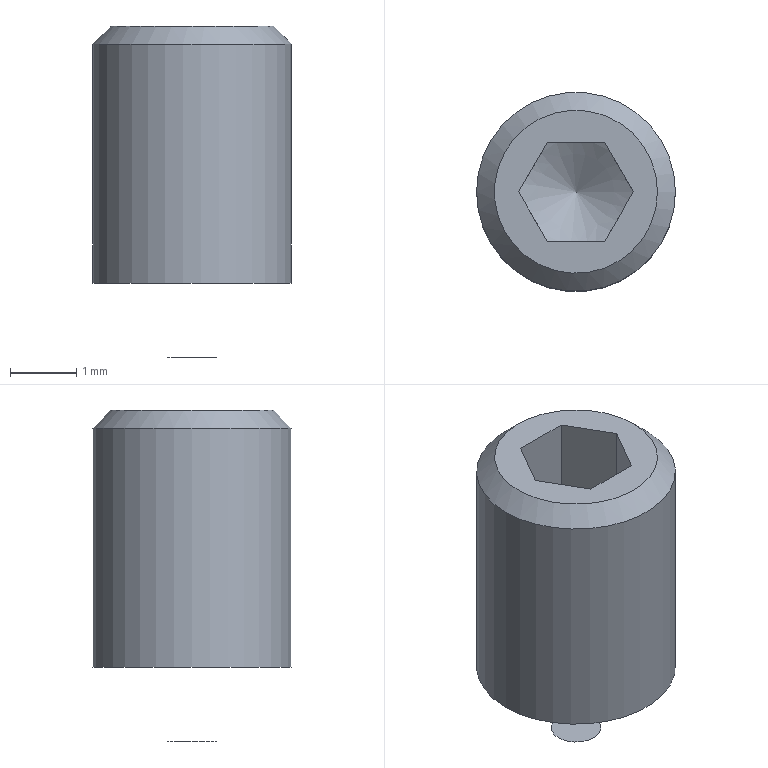Part | NX | features BREP 1, DATUM_CSYS 1 | 1 solid | 12 faces | box 3 x 3 x 5 mm | volume 26.266 mm3 | plane 8 | cone 3 | cylinder 1 | commonest cylinder face diameters 3 x1
STEP:
#1=CARTESIAN_POINT('',(0.866,0.,0.));
#2=VERTEX_POINT('',#1);
#3=CARTESIAN_POINT('',(0.866,0.,-2.));
#4=VERTEX_POINT('',#3);
#5=CARTESIAN_POINT('',(0.866,0.,0.));
#6=DIRECTION('',(0.,0.,-1.));
#7=VECTOR('',#6,1000.);
#8=LINE('',#5,#7);
#9=EDGE_CURVE('',#2,#4,#8,.T.);
#10=ORIENTED_EDGE('',*,*,#9,.T.);
#11=CARTESIAN_POINT('',(0.433,-0.75,-2.));
#12=VERTEX_POINT('',#11);
#13=CARTESIAN_POINT('',(0.866,0.,-2.));
#14=CARTESIAN_POINT('',(0.6495,-0.375,-2.125));
#15=CARTESIAN_POINT('',(0.433,-0.75,-2.));
#16=(BOUNDED_CURVE()B_SPLINE_CURVE(2,(#13,#14,#15),.UNSPECIFIED.,.F.,.F.)B_SPLINE_CURVE_WITH_KNOTS((3,3),(0.,1.),.PIECEWISE_BEZIER_KNOTS.)CURVE()GEOMETRIC_REPRESENTATION_ITEM()RATIONAL_B_SPLINE_CURVE((1.,1.155,1.))REPRESENTATION_ITEM(''));
#17=EDGE_CURVE('',#4,#12,#16,.T.);
#18=ORIENTED_EDGE('',*,*,#17,.T.);
#19=CARTESIAN_POINT('',(0.433,-0.75,0.));
#20=VERTEX_POINT('',#19);
#21=CARTESIAN_POINT('',(0.433,-0.75,0.));
#22=DIRECTION('',(0.,0.,-1.));
#23=VECTOR('',#22,1000.);
#24=LINE('',#21,#23);
#25=EDGE_CURVE('',#20,#12,#24,.T.);
#26=ORIENTED_EDGE('',*,*,#25,.F.);
#27=CARTESIAN_POINT('',(0.866,0.,0.));
#28=DIRECTION('',(-0.5,-0.866,0.));
#29=VECTOR('',#28,1000.);
#30=LINE('',#27,#29);
#31=EDGE_CURVE('',#2,#20,#30,.T.);
#32=ORIENTED_EDGE('',*,*,#31,.F.);
#33=EDGE_LOOP('',(#10,#18,#26,#32));
#34=FACE_BOUND('',#33,.T.);
#35=CARTESIAN_POINT('',(0.6495,-0.375,-1.1));
#36=DIRECTION('',(0.866,-0.5,0.));
#37=DIRECTION('',(0.5,0.866,0.));
#38=AXIS2_PLACEMENT_3D('',#35,#36,#37);
#39=PLANE('',#38);
#40=ADVANCED_FACE('',(#34),#39,.F.);
#41=ORIENTED_EDGE('',*,*,#25,.T.);
#42=CARTESIAN_POINT('',(-0.433,-0.75,-2.));
#43=VERTEX_POINT('',#42);
#44=CARTESIAN_POINT('',(0.433,-0.75,-2.));
#45=CARTESIAN_POINT('',(0.,-0.75,-2.125));
#46=CARTESIAN_POINT('',(-0.433,-0.75,-2.));
#47=(BOUNDED_CURVE()B_SPLINE_CURVE(2,(#44,#45,#46),.UNSPECIFIED.,.F.,.F.)B_SPLINE_CURVE_WITH_KNOTS((3,3),(0.,1.),.PIECEWISE_BEZIER_KNOTS.)CURVE()GEOMETRIC_REPRESENTATION_ITEM()RATIONAL_B_SPLINE_CURVE((1.,1.155,1.))REPRESENTATION_ITEM(''));
#48=EDGE_CURVE('',#12,#43,#47,.T.);
#49=ORIENTED_EDGE('',*,*,#48,.T.);
#50=CARTESIAN_POINT('',(-0.433,-0.75,0.));
#51=VERTEX_POINT('',#50);
#52=CARTESIAN_POINT('',(-0.433,-0.75,0.));
#53=DIRECTION('',(0.,0.,-1.));
#54=VECTOR('',#53,1000.);
#55=LINE('',#52,#54);
#56=EDGE_CURVE('',#51,#43,#55,.T.);
#57=ORIENTED_EDGE('',*,*,#56,.F.);
#58=CARTESIAN_POINT('',(0.433,-0.75,0.));
#59=DIRECTION('',(-1.,0.,0.));
#60=VECTOR('',#59,1000.);
#61=LINE('',#58,#60);
#62=EDGE_CURVE('',#20,#51,#61,.T.);
#63=ORIENTED_EDGE('',*,*,#62,.F.);
#64=EDGE_LOOP('',(#41,#49,#57,#63));
#65=FACE_BOUND('',#64,.T.);
#66=CARTESIAN_POINT('',(0.,-0.75,-1.1));
#67=DIRECTION('',(0.,-1.,0.));
#68=DIRECTION('',(1.,0.,0.));
#69=AXIS2_PLACEMENT_3D('',#66,#67,#68);
#70=PLANE('',#69);
#71=ADVANCED_FACE('',(#65),#70,.F.);
#72=ORIENTED_EDGE('',*,*,#56,.T.);
#73=CARTESIAN_POINT('',(-0.866,0.,-2.));
#74=VERTEX_POINT('',#73);
#75=CARTESIAN_POINT('',(-0.433,-0.75,-2.));
#76=CARTESIAN_POINT('',(-0.6495,-0.375,-2.125));
#77=CARTESIAN_POINT('',(-0.866,0.,-2.));
#78=(BOUNDED_CURVE()B_SPLINE_CURVE(2,(#75,#76,#77),.UNSPECIFIED.,.F.,.F.)B_SPLINE_CURVE_WITH_KNOTS((3,3),(0.,1.),.PIECEWISE_BEZIER_KNOTS.)CURVE()GEOMETRIC_REPRESENTATION_ITEM()RATIONAL_B_SPLINE_CURVE((1.,1.155,1.))REPRESENTATION_ITEM(''));
#79=EDGE_CURVE('',#43,#74,#78,.T.);
#80=ORIENTED_EDGE('',*,*,#79,.T.);
#81=CARTESIAN_POINT('',(-0.866,0.,0.));
#82=VERTEX_POINT('',#81);
#83=CARTESIAN_POINT('',(-0.866,0.,0.));
#84=DIRECTION('',(0.,0.,-1.));
#85=VECTOR('',#84,1000.);
#86=LINE('',#83,#85);
#87=EDGE_CURVE('',#82,#74,#86,.T.);
#88=ORIENTED_EDGE('',*,*,#87,.F.);
#89=CARTESIAN_POINT('',(-0.433,-0.75,0.));
#90=DIRECTION('',(-0.5,0.866,0.));
#91=VECTOR('',#90,1000.);
#92=LINE('',#89,#91);
#93=EDGE_CURVE('',#51,#82,#92,.T.);
#94=ORIENTED_EDGE('',*,*,#93,.F.);
#95=EDGE_LOOP('',(#72,#80,#88,#94));
#96=FACE_BOUND('',#95,.T.);
#97=CARTESIAN_POINT('',(-0.6495,-0.375,-1.1));
#98=DIRECTION('',(-0.866,-0.5,0.));
#99=DIRECTION('',(0.5,-0.866,0.));
#100=AXIS2_PLACEMENT_3D('',#97,#98,#99);
#101=PLANE('',#100);
#102=ADVANCED_FACE('',(#96),#101,.F.);
#103=ORIENTED_EDGE('',*,*,#87,.T.);
#104=CARTESIAN_POINT('',(-0.433,0.75,-2.));
#105=VERTEX_POINT('',#104);
#106=CARTESIAN_POINT('',(-0.866,0.,-2.));
#107=CARTESIAN_POINT('',(-0.6495,0.375,-2.125));
#108=CARTESIAN_POINT('',(-0.433,0.75,-2.));
#109=(BOUNDED_CURVE()B_SPLINE_CURVE(2,(#106,#107,#108),.UNSPECIFIED.,.F.,.F.)B_SPLINE_CURVE_WITH_KNOTS((3,3),(0.,1.),.PIECEWISE_BEZIER_KNOTS.)CURVE()GEOMETRIC_REPRESENTATION_ITEM()RATIONAL_B_SPLINE_CURVE((1.,1.155,1.))REPRESENTATION_ITEM(''));
#110=EDGE_CURVE('',#74,#105,#109,.T.);
#111=ORIENTED_EDGE('',*,*,#110,.T.);
#112=CARTESIAN_POINT('',(-0.433,0.75,0.));
#113=VERTEX_POINT('',#112);
#114=CARTESIAN_POINT('',(-0.433,0.75,0.));
#115=DIRECTION('',(0.,0.,-1.));
#116=VECTOR('',#115,1000.);
#117=LINE('',#114,#116);
#118=EDGE_CURVE('',#113,#105,#117,.T.);
#119=ORIENTED_EDGE('',*,*,#118,.F.);
#120=CARTESIAN_POINT('',(-0.866,0.,0.));
#121=DIRECTION('',(0.5,0.866,0.));
#122=VECTOR('',#121,1000.);
#123=LINE('',#120,#122);
#124=EDGE_CURVE('',#82,#113,#123,.T.);
#125=ORIENTED_EDGE('',*,*,#124,.F.);
#126=EDGE_LOOP('',(#103,#111,#119,#125));
#127=FACE_BOUND('',#126,.T.);
#128=CARTESIAN_POINT('',(-0.6495,0.375,-1.1));
#129=DIRECTION('',(-0.866,0.5,0.));
#130=DIRECTION('',(-0.5,-0.866,0.));
#131=AXIS2_PLACEMENT_3D('',#128,#129,#130);
#132=PLANE('',#131);
#133=ADVANCED_FACE('',(#127),#132,.F.);
#134=ORIENTED_EDGE('',*,*,#118,.T.);
#135=CARTESIAN_POINT('',(0.433,0.75,-2.));
#136=VERTEX_POINT('',#135);
#137=CARTESIAN_POINT('',(-0.433,0.75,-2.));
#138=CARTESIAN_POINT('',(0.,0.75,-2.125));
#139=CARTESIAN_POINT('',(0.433,0.75,-2.));
#140=(BOUNDED_CURVE()B_SPLINE_CURVE(2,(#137,#138,#139),.UNSPECIFIED.,.F.,.F.)B_SPLINE_CURVE_WITH_KNOTS((3,3),(0.,1.),.PIECEWISE_BEZIER_KNOTS.)CURVE()GEOMETRIC_REPRESENTATION_ITEM()RATIONAL_B_SPLINE_CURVE((1.,1.155,1.))REPRESENTATION_ITEM(''));
#141=EDGE_CURVE('',#105,#136,#140,.T.);
#142=ORIENTED_EDGE('',*,*,#141,.T.);
#143=CARTESIAN_POINT('',(0.433,0.75,0.));
#144=VERTEX_POINT('',#143);
#145=CARTESIAN_POINT('',(0.433,0.75,0.));
#146=DIRECTION('',(0.,0.,-1.));
#147=VECTOR('',#146,1000.);
#148=LINE('',#145,#147);
#149=EDGE_CURVE('',#144,#136,#148,.T.);
#150=ORIENTED_EDGE('',*,*,#149,.F.);
#151=CARTESIAN_POINT('',(-0.433,0.75,0.));
#152=DIRECTION('',(1.,0.,0.));
#153=VECTOR('',#152,1000.);
#154=LINE('',#151,#153);
#155=EDGE_CURVE('',#113,#144,#154,.T.);
#156=ORIENTED_EDGE('',*,*,#155,.F.);
#157=EDGE_LOOP('',(#134,#142,#150,#156));
#158=FACE_BOUND('',#157,.T.);
#159=CARTESIAN_POINT('',(0.,0.75,-1.1));
#160=DIRECTION('',(0.,1.,0.));
#161=DIRECTION('',(-1.,0.,0.));
#162=AXIS2_PLACEMENT_3D('',#159,#160,#161);
#163=PLANE('',#162);
#164=ADVANCED_FACE('',(#158),#163,.F.);
#165=ORIENTED_EDGE('',*,*,#149,.T.);
#166=CARTESIAN_POINT('',(0.433,0.75,-2.));
#167=CARTESIAN_POINT('',(0.6495,0.375,-2.125));
#168=CARTESIAN_POINT('',(0.866,0.,-2.));
#169=(BOUNDED_CURVE()B_SPLINE_CURVE(2,(#166,#167,#168),.UNSPECIFIED.,.F.,.F.)B_SPLINE_CURVE_WITH_KNOTS((3,3),(0.,1.),.PIECEWISE_BEZIER_KNOTS.)CURVE()GEOMETRIC_REPRESENTATION_ITEM()RATIONAL_B_SPLINE_CURVE((1.,1.155,1.))REPRESENTATION_ITEM(''));
#170=EDGE_CURVE('',#136,#4,#169,.T.);
#171=ORIENTED_EDGE('',*,*,#170,.T.);
#172=ORIENTED_EDGE('',*,*,#9,.F.);
#173=CARTESIAN_POINT('',(0.433,0.75,0.));
#174=DIRECTION('',(0.5,-0.866,0.));
#175=VECTOR('',#174,1000.);
#176=LINE('',#173,#175);
#177=EDGE_CURVE('',#144,#2,#176,.T.);
#178=ORIENTED_EDGE('',*,*,#177,.F.);
#179=EDGE_LOOP('',(#165,#171,#172,#178));
#180=FACE_BOUND('',#179,.T.);
#181=CARTESIAN_POINT('',(0.6495,0.375,-1.1));
#182=DIRECTION('',(0.866,0.5,0.));
#183=DIRECTION('',(-0.5,0.866,0.));
#184=AXIS2_PLACEMENT_3D('',#181,#182,#183);
#185=PLANE('',#184);
#186=ADVANCED_FACE('',(#180),#185,.F.);
#187=CARTESIAN_POINT('',(0.,0.,-2.5));
#188=VERTEX_POINT('',#187);
#189=CARTESIAN_POINT('',(0.866,0.,-2.));
#190=DIRECTION('',(-0.866,0.,-0.5));
#191=VECTOR('',#190,1000.);
#192=LINE('',#189,#191);
#193=EDGE_CURVE('',#4,#188,#192,.T.);
#194=ORIENTED_EDGE('',*,*,#193,.T.);
#195=ORIENTED_EDGE('',*,*,#193,.F.);
#196=ORIENTED_EDGE('',*,*,#170,.F.);
#197=ORIENTED_EDGE('',*,*,#141,.F.);
#198=ORIENTED_EDGE('',*,*,#110,.F.);
#199=ORIENTED_EDGE('',*,*,#79,.F.);
#200=ORIENTED_EDGE('',*,*,#48,.F.);
#201=ORIENTED_EDGE('',*,*,#17,.F.);
#202=EDGE_LOOP('',(#194,#195,#196,#197,#198,#199,#200,#201));
#203=FACE_BOUND('',#202,.T.);
#204=CARTESIAN_POINT('',(0.,0.,-2.5));
#205=DIRECTION('',(0.,0.,1.));
#206=DIRECTION('',(-1.,0.,0.));
#207=AXIS2_PLACEMENT_3D('',#204,#205,#206);
#208=CONICAL_SURFACE('',#207,0.,1.047);
#209=ADVANCED_FACE('',(#203),#208,.F.);
#210=CARTESIAN_POINT('',(1.229,0.,0.));
#211=VERTEX_POINT('',#210);
#212=CARTESIAN_POINT('',(0.,0.,0.));
#213=DIRECTION('',(0.,0.,-1.));
#214=DIRECTION('',(1.,0.,0.));
#215=AXIS2_PLACEMENT_3D('',#212,#213,#214);
#216=CIRCLE('',#215,1.229);
#217=EDGE_CURVE('',#211,#211,#216,.T.);
#218=ORIENTED_EDGE('',*,*,#217,.F.);
#219=EDGE_LOOP('',(#218));
#220=FACE_BOUND('',#219,.T.);
#221=ORIENTED_EDGE('',*,*,#93,.T.);
#222=ORIENTED_EDGE('',*,*,#124,.T.);
#223=ORIENTED_EDGE('',*,*,#155,.T.);
#224=ORIENTED_EDGE('',*,*,#177,.T.);
#225=ORIENTED_EDGE('',*,*,#31,.T.);
#226=ORIENTED_EDGE('',*,*,#62,.T.);
#227=EDGE_LOOP('',(#221,#222,#223,#224,#225,#226));
#228=FACE_BOUND('',#227,.T.);
#229=CARTESIAN_POINT('',(0.,0.,0.));
#230=DIRECTION('',(0.,0.,1.));
#231=DIRECTION('',(-1.,0.,0.));
#232=AXIS2_PLACEMENT_3D('',#229,#230,#231);
#233=PLANE('',#232);
#234=ADVANCED_FACE('',(#220,#228),#233,.T.);
#235=CARTESIAN_POINT('',(1.5,0.,-0.2706));
#236=VERTEX_POINT('',#235);
#237=CARTESIAN_POINT('',(1.5,0.,-0.2706));
#238=DIRECTION('',(-0.7071,0.,0.7071));
#239=VECTOR('',#238,1000.);
#240=LINE('',#237,#239);
#241=EDGE_CURVE('',#236,#211,#240,.T.);
#242=ORIENTED_EDGE('',*,*,#241,.T.);
#243=ORIENTED_EDGE('',*,*,#217,.T.);
#244=ORIENTED_EDGE('',*,*,#241,.F.);
#245=CARTESIAN_POINT('',(0.,0.,-0.2706));
#246=DIRECTION('',(0.,0.,-1.));
#247=DIRECTION('',(1.,0.,0.));
#248=AXIS2_PLACEMENT_3D('',#245,#246,#247);
#249=CIRCLE('',#248,1.5);
#250=EDGE_CURVE('',#236,#236,#249,.T.);
#251=ORIENTED_EDGE('',*,*,#250,.F.);
#252=EDGE_LOOP('',(#242,#243,#244,#251));
#253=FACE_BOUND('',#252,.T.);
#254=CARTESIAN_POINT('',(0.,0.,0.));
#255=DIRECTION('',(0.,0.,-1.));
#256=DIRECTION('',(-1.,0.,0.));
#257=AXIS2_PLACEMENT_3D('',#254,#255,#256);
#258=CONICAL_SURFACE('',#257,1.229,0.7854);
#259=ADVANCED_FACE('',(#253),#258,.T.);
#260=CARTESIAN_POINT('',(1.5,0.,-3.875));
#261=VERTEX_POINT('',#260);
#262=CARTESIAN_POINT('',(1.5,0.,-3.875));
#263=DIRECTION('',(0.,0.,1.));
#264=VECTOR('',#263,1000.);
#265=LINE('',#262,#264);
#266=EDGE_CURVE('',#261,#236,#265,.T.);
#267=ORIENTED_EDGE('',*,*,#266,.T.);
#268=ORIENTED_EDGE('',*,*,#250,.T.);
#269=ORIENTED_EDGE('',*,*,#266,.F.);
#270=CARTESIAN_POINT('',(0.,0.,-3.875));
#271=DIRECTION('',(0.,0.,-1.));
#272=DIRECTION('',(1.,0.,0.));
#273=AXIS2_PLACEMENT_3D('',#270,#271,#272);
#274=CIRCLE('',#273,1.5);
#275=EDGE_CURVE('',#261,#261,#274,.T.);
#276=ORIENTED_EDGE('',*,*,#275,.F.);
#277=EDGE_LOOP('',(#267,#268,#269,#276));
#278=FACE_BOUND('',#277,.T.);
#279=CARTESIAN_POINT('',(0.,0.,-3.875));
#280=DIRECTION('',(0.,0.,1.));
#281=DIRECTION('',(-1.,0.,0.));
#282=AXIS2_PLACEMENT_3D('',#279,#280,#281);
#283=CYLINDRICAL_SURFACE('',#282,1.5);
#284=ADVANCED_FACE('',(#278),#283,.T.);
#285=CARTESIAN_POINT('',(0.375,0.,-5.));
#286=VERTEX_POINT('',#285);
#287=CARTESIAN_POINT('',(0.375,0.,-5.));
#288=DIRECTION('',(0.7071,0.,0.7071));
#289=VECTOR('',#288,1000.);
#290=LINE('',#287,#289);
#291=EDGE_CURVE('',#286,#261,#290,.T.);
#292=ORIENTED_EDGE('',*,*,#291,.T.);
#293=ORIENTED_EDGE('',*,*,#275,.T.);
#294=ORIENTED_EDGE('',*,*,#291,.F.);
#295=CARTESIAN_POINT('',(0.,0.,-5.));
#296=DIRECTION('',(0.,0.,-1.));
#297=DIRECTION('',(1.,0.,0.));
#298=AXIS2_PLACEMENT_3D('',#295,#296,#297);
#299=CIRCLE('',#298,0.375);
#300=EDGE_CURVE('',#286,#286,#299,.T.);
#301=ORIENTED_EDGE('',*,*,#300,.F.);
#302=EDGE_LOOP('',(#292,#293,#294,#301));
#303=FACE_BOUND('',#302,.T.);
#304=CARTESIAN_POINT('',(0.,0.,-5.));
#305=DIRECTION('',(0.,0.,1.));
#306=DIRECTION('',(-1.,0.,0.));
#307=AXIS2_PLACEMENT_3D('',#304,#305,#306);
#308=CONICAL_SURFACE('',#307,0.375,0.7854);
#309=ADVANCED_FACE('',(#303),#308,.T.);
#310=ORIENTED_EDGE('',*,*,#300,.T.);
#311=EDGE_LOOP('',(#310));
#312=FACE_BOUND('',#311,.T.);
#313=CARTESIAN_POINT('',(0.,0.,-5.));
#314=DIRECTION('',(0.,0.,-1.));
#315=DIRECTION('',(-1.,0.,0.));
#316=AXIS2_PLACEMENT_3D('',#313,#314,#315);
#317=PLANE('',#316);
#318=ADVANCED_FACE('',(#312),#317,.T.);
#319=CLOSED_SHELL('',(#40,#71,#102,#133,#164,#186,#209,#234,#259,#284,#309,#318));
#320=MANIFOLD_SOLID_BREP('',#319);
#321=(LENGTH_UNIT()NAMED_UNIT(*)SI_UNIT(.MILLI.,.METRE.));
#322=UNCERTAINTY_MEASURE_WITH_UNIT(LENGTH_MEASURE(0.00001),#321,'','');
#323=(NAMED_UNIT(*)PLANE_ANGLE_UNIT()SI_UNIT($,.RADIAN.));
#324=(NAMED_UNIT(*)SI_UNIT($,.STERADIAN.)SOLID_ANGLE_UNIT());
#325=(GEOMETRIC_REPRESENTATION_CONTEXT(3)GLOBAL_UNCERTAINTY_ASSIGNED_CONTEXT((#322))GLOBAL_UNIT_ASSIGNED_CONTEXT((#321,#323,#324))REPRESENTATION_CONTEXT('',''));
#326=ADVANCED_BREP_SHAPE_REPRESENTATION('',(#320),#325);